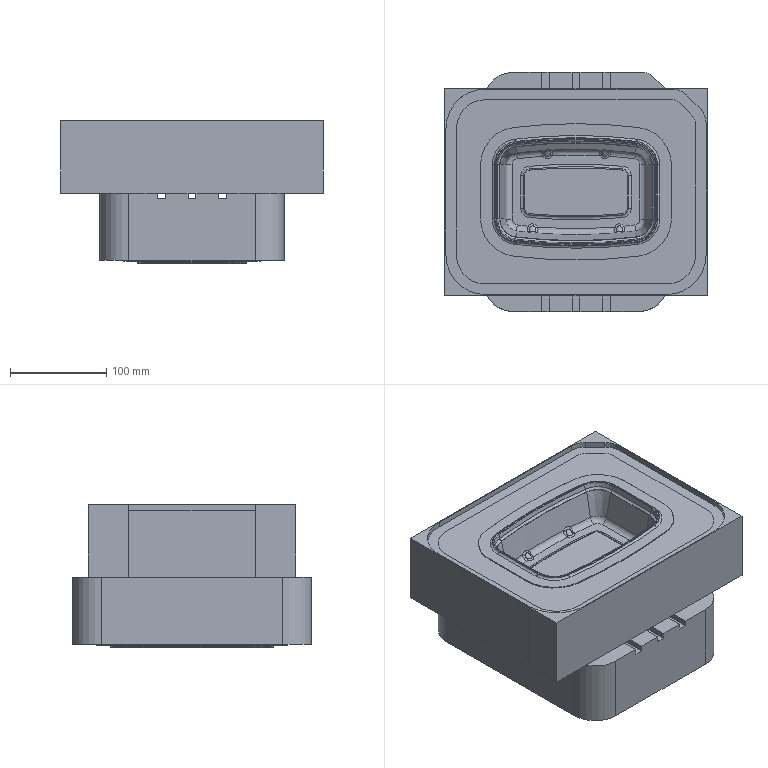Part | 4 solids | 566 faces | box 272.387 x 248.388 x 148.5 mm | volume 6223544 mm3 | plane 211 | cylinder 189 | torus 92 | spline 54 | cone 20 | commonest cylinder face diameters 2 x44 8 x44 60 x9 1 x8 9.958 x8 77.811 x8